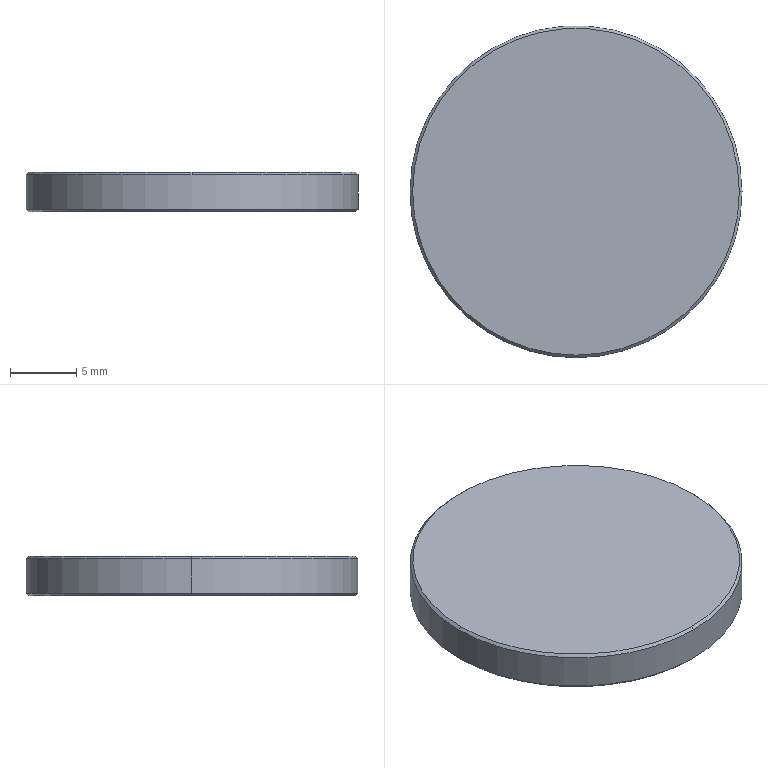Part | STEP file | TCHK-2D-D30-BB-TC-30X3.stp.STEP | 1 solid | 10 faces | box 25 x 25 x 3 mm | volume 1469 mm3 | cone 6 | plane 2 | cylinder 2 | commonest cylinder face diameters 25 x2
STEP:
#1=CARTESIAN_POINT('',(-12.3,0.,0.000000292));
#2=VERTEX_POINT('',#1);
#3=CARTESIAN_POINT('',(12.3,0.,0.000000292));
#4=VERTEX_POINT('',#3);
#5=CARTESIAN_POINT('',(0.,0.,0.000000292));
#6=DIRECTION('',(0.,0.,-1.));
#7=DIRECTION('',(-1.,0.,0.));
#8=AXIS2_PLACEMENT_3D('',#5,#6,#7);
#9=CIRCLE('',#8,12.3);
#10=EDGE_CURVE('',#2,#4,#9,.T.);
#11=ORIENTED_EDGE('',*,*,#10,.T.);
#12=CARTESIAN_POINT('',(0.,-12.3,0.000000292));
#13=VERTEX_POINT('',#12);
#14=CARTESIAN_POINT('',(0.,0.,0.000000292));
#15=DIRECTION('',(0.,0.,-1.));
#16=DIRECTION('',(1.,0.,0.));
#17=AXIS2_PLACEMENT_3D('',#14,#15,#16);
#18=CIRCLE('',#17,12.3);
#19=EDGE_CURVE('',#4,#13,#18,.T.);
#20=ORIENTED_EDGE('',*,*,#19,.T.);
#21=CARTESIAN_POINT('',(0.,0.,0.000000292));
#22=DIRECTION('',(0.,0.,-1.));
#23=DIRECTION('',(1.,0.,0.));
#24=AXIS2_PLACEMENT_3D('',#21,#22,#23);
#25=CIRCLE('',#24,12.3);
#26=EDGE_CURVE('',#13,#2,#25,.T.);
#27=ORIENTED_EDGE('',*,*,#26,.T.);
#28=EDGE_LOOP('',(#11,#20,#27));
#29=FACE_OUTER_BOUND('',#28,.T.);
#30=CARTESIAN_POINT('',(0.,0.,0.));
#31=DIRECTION('',(0.,0.,1.));
#32=DIRECTION('',(1.,0.,0.));
#33=AXIS2_PLACEMENT_3D('',#30,#31,#32);
#34=PLANE('',#33);
#35=ADVANCED_FACE('',(#29),#34,.F.);
#36=CARTESIAN_POINT('',(0.,-12.5,0.2));
#37=VERTEX_POINT('',#36);
#38=CARTESIAN_POINT('',(0.,-12.4,0.1));
#39=DIRECTION('',(0.,-0.7071,0.7071));
#40=VECTOR('',#39,1000.);
#41=LINE('',#38,#40);
#42=EDGE_CURVE('',#13,#37,#41,.T.);
#43=ORIENTED_EDGE('',*,*,#42,.F.);
#44=ORIENTED_EDGE('',*,*,#19,.F.);
#45=CARTESIAN_POINT('',(12.5,0.,0.2));
#46=VERTEX_POINT('',#45);
#47=CARTESIAN_POINT('',(12.3,0.000000002,0.000000547));
#48=DIRECTION('',(0.7071,-0.000000002,0.7071));
#49=VECTOR('',#48,1000.);
#50=LINE('',#47,#49);
#51=EDGE_CURVE('',#4,#46,#50,.T.);
#52=ORIENTED_EDGE('',*,*,#51,.T.);
#53=CARTESIAN_POINT('',(0.,0.,0.2));
#54=DIRECTION('',(0.,0.,-1.));
#55=DIRECTION('',(1.,0.,0.));
#56=AXIS2_PLACEMENT_3D('',#53,#54,#55);
#57=CIRCLE('',#56,12.5);
#58=EDGE_CURVE('',#46,#37,#57,.T.);
#59=ORIENTED_EDGE('',*,*,#58,.T.);
#60=EDGE_LOOP('',(#43,#44,#52,#59));
#61=FACE_OUTER_BOUND('',#60,.T.);
#62=CARTESIAN_POINT('',(0.,0.,0.1));
#63=DIRECTION('',(0.,0.,1.));
#64=DIRECTION('',(0.,-1.,0.));
#65=AXIS2_PLACEMENT_3D('',#62,#63,#64);
#66=CONICAL_SURFACE('',#65,12.4,0.7854);
#67=ADVANCED_FACE('',(#61),#66,.T.);
#68=CARTESIAN_POINT('',(-12.5,0.,0.2));
#69=VERTEX_POINT('',#68);
#70=CARTESIAN_POINT('',(-12.3,-0.000000002,0.000000547));
#71=DIRECTION('',(-0.7071,0.000000002,0.7071));
#72=VECTOR('',#71,1000.);
#73=LINE('',#70,#72);
#74=EDGE_CURVE('',#2,#69,#73,.T.);
#75=ORIENTED_EDGE('',*,*,#74,.T.);
#76=CARTESIAN_POINT('',(0.,0.,0.2));
#77=DIRECTION('',(0.,0.,-1.));
#78=DIRECTION('',(-1.,0.,0.));
#79=AXIS2_PLACEMENT_3D('',#76,#77,#78);
#80=CIRCLE('',#79,12.5);
#81=EDGE_CURVE('',#69,#46,#80,.T.);
#82=ORIENTED_EDGE('',*,*,#81,.T.);
#83=ORIENTED_EDGE('',*,*,#51,.F.);
#84=ORIENTED_EDGE('',*,*,#10,.F.);
#85=EDGE_LOOP('',(#75,#82,#83,#84));
#86=FACE_OUTER_BOUND('',#85,.T.);
#87=CARTESIAN_POINT('',(0.,0.,0.1));
#88=DIRECTION('',(0.,0.,1.));
#89=DIRECTION('',(0.,-1.,0.));
#90=AXIS2_PLACEMENT_3D('',#87,#88,#89);
#91=CONICAL_SURFACE('',#90,12.4,0.7854);
#92=ADVANCED_FACE('',(#86),#91,.T.);
#93=CARTESIAN_POINT('',(12.5,0.,2.8));
#94=VERTEX_POINT('',#93);
#95=CARTESIAN_POINT('',(12.5,0.000000001,0.2));
#96=DIRECTION('',(0.,0.,1.));
#97=VECTOR('',#96,1000.);
#98=LINE('',#95,#97);
#99=EDGE_CURVE('',#46,#94,#98,.T.);
#100=ORIENTED_EDGE('',*,*,#99,.F.);
#101=ORIENTED_EDGE('',*,*,#81,.F.);
#102=CARTESIAN_POINT('',(-12.5,0.,2.8));
#103=VERTEX_POINT('',#102);
#104=CARTESIAN_POINT('',(-12.5,-0.000000001,0.2));
#105=DIRECTION('',(0.,0.,1.));
#106=VECTOR('',#105,1000.);
#107=LINE('',#104,#106);
#108=EDGE_CURVE('',#69,#103,#107,.T.);
#109=ORIENTED_EDGE('',*,*,#108,.T.);
#110=CARTESIAN_POINT('',(0.,0.,2.8));
#111=DIRECTION('',(0.,0.,1.));
#112=DIRECTION('',(1.,0.,0.));
#113=AXIS2_PLACEMENT_3D('',#110,#111,#112);
#114=CIRCLE('',#113,12.5);
#115=EDGE_CURVE('',#94,#103,#114,.T.);
#116=ORIENTED_EDGE('',*,*,#115,.F.);
#117=EDGE_LOOP('',(#100,#101,#109,#116));
#118=FACE_OUTER_BOUND('',#117,.T.);
#119=CARTESIAN_POINT('',(0.,0.,0.));
#120=DIRECTION('',(0.,0.,1.));
#121=DIRECTION('',(1.,0.,0.));
#122=AXIS2_PLACEMENT_3D('',#119,#120,#121);
#123=CYLINDRICAL_SURFACE('',#122,12.5);
#124=ADVANCED_FACE('',(#118),#123,.T.);
#125=CARTESIAN_POINT('',(12.3,0.,3.));
#126=VERTEX_POINT('',#125);
#127=CARTESIAN_POINT('',(12.3,0.000000002,3.));
#128=DIRECTION('',(0.7071,-0.000000002,-0.7071));
#129=VECTOR('',#128,1000.);
#130=LINE('',#127,#129);
#131=EDGE_CURVE('',#126,#94,#130,.T.);
#132=ORIENTED_EDGE('',*,*,#131,.T.);
#133=ORIENTED_EDGE('',*,*,#115,.T.);
#134=CARTESIAN_POINT('',(-12.3,0.,3.));
#135=VERTEX_POINT('',#134);
#136=CARTESIAN_POINT('',(-12.3,-0.000000002,3.));
#137=DIRECTION('',(-0.7071,0.000000002,-0.7071));
#138=VECTOR('',#137,1000.);
#139=LINE('',#136,#138);
#140=EDGE_CURVE('',#135,#103,#139,.T.);
#141=ORIENTED_EDGE('',*,*,#140,.F.);
#142=CARTESIAN_POINT('',(0.,0.,3.));
#143=DIRECTION('',(0.,0.,1.));
#144=DIRECTION('',(1.,0.,0.));
#145=AXIS2_PLACEMENT_3D('',#142,#143,#144);
#146=CIRCLE('',#145,12.3);
#147=EDGE_CURVE('',#126,#135,#146,.T.);
#148=ORIENTED_EDGE('',*,*,#147,.F.);
#149=EDGE_LOOP('',(#132,#133,#141,#148));
#150=FACE_OUTER_BOUND('',#149,.T.);
#151=CARTESIAN_POINT('',(0.,0.,2.9));
#152=DIRECTION('',(0.,0.,-1.));
#153=DIRECTION('',(0.,-1.,0.));
#154=AXIS2_PLACEMENT_3D('',#151,#152,#153);
#155=CONICAL_SURFACE('',#154,12.4,0.7854);
#156=ADVANCED_FACE('',(#150),#155,.T.);
#157=ORIENTED_EDGE('',*,*,#147,.T.);
#158=CARTESIAN_POINT('',(0.,-12.3,3.));
#159=VERTEX_POINT('',#158);
#160=CARTESIAN_POINT('',(0.,0.,3.));
#161=DIRECTION('',(0.,0.,1.));
#162=DIRECTION('',(-1.,0.,0.));
#163=AXIS2_PLACEMENT_3D('',#160,#161,#162);
#164=CIRCLE('',#163,12.3);
#165=EDGE_CURVE('',#135,#159,#164,.T.);
#166=ORIENTED_EDGE('',*,*,#165,.T.);
#167=CARTESIAN_POINT('',(0.,0.,3.));
#168=DIRECTION('',(0.,0.,1.));
#169=DIRECTION('',(-1.,0.,0.));
#170=AXIS2_PLACEMENT_3D('',#167,#168,#169);
#171=CIRCLE('',#170,12.3);
#172=EDGE_CURVE('',#159,#126,#171,.T.);
#173=ORIENTED_EDGE('',*,*,#172,.T.);
#174=EDGE_LOOP('',(#157,#166,#173));
#175=FACE_OUTER_BOUND('',#174,.T.);
#176=CARTESIAN_POINT('',(0.,0.,3.));
#177=DIRECTION('',(0.,0.,1.));
#178=DIRECTION('',(1.,0.,0.));
#179=AXIS2_PLACEMENT_3D('',#176,#177,#178);
#180=PLANE('',#179);
#181=ADVANCED_FACE('',(#175),#180,.T.);
#182=CARTESIAN_POINT('',(0.,-12.5,2.8));
#183=VERTEX_POINT('',#182);
#184=CARTESIAN_POINT('',(0.,-12.4,2.9));
#185=DIRECTION('',(0.,-0.7071,-0.7071));
#186=VECTOR('',#185,1000.);
#187=LINE('',#184,#186);
#188=EDGE_CURVE('',#159,#183,#187,.T.);
#189=ORIENTED_EDGE('',*,*,#188,.F.);
#190=ORIENTED_EDGE('',*,*,#165,.F.);
#191=ORIENTED_EDGE('',*,*,#140,.T.);
#192=CARTESIAN_POINT('',(0.,0.,2.8));
#193=DIRECTION('',(0.,0.,1.));
#194=DIRECTION('',(-1.,0.,0.));
#195=AXIS2_PLACEMENT_3D('',#192,#193,#194);
#196=CIRCLE('',#195,12.5);
#197=EDGE_CURVE('',#103,#183,#196,.T.);
#198=ORIENTED_EDGE('',*,*,#197,.T.);
#199=EDGE_LOOP('',(#189,#190,#191,#198));
#200=FACE_OUTER_BOUND('',#199,.T.);
#201=CARTESIAN_POINT('',(0.,0.,2.9));
#202=DIRECTION('',(0.,0.,-1.));
#203=DIRECTION('',(0.,-1.,0.));
#204=AXIS2_PLACEMENT_3D('',#201,#202,#203);
#205=CONICAL_SURFACE('',#204,12.4,0.7854);
#206=ADVANCED_FACE('',(#200),#205,.T.);
#207=ORIENTED_EDGE('',*,*,#108,.F.);
#208=CARTESIAN_POINT('',(0.,0.,0.2));
#209=DIRECTION('',(0.,0.,-1.));
#210=DIRECTION('',(1.,0.,0.));
#211=AXIS2_PLACEMENT_3D('',#208,#209,#210);
#212=CIRCLE('',#211,12.5);
#213=EDGE_CURVE('',#37,#69,#212,.T.);
#214=ORIENTED_EDGE('',*,*,#213,.F.);
#215=ORIENTED_EDGE('',*,*,#58,.F.);
#216=ORIENTED_EDGE('',*,*,#99,.T.);
#217=CARTESIAN_POINT('',(0.,0.,2.8));
#218=DIRECTION('',(0.,0.,1.));
#219=DIRECTION('',(-1.,0.,0.));
#220=AXIS2_PLACEMENT_3D('',#217,#218,#219);
#221=CIRCLE('',#220,12.5);
#222=EDGE_CURVE('',#183,#94,#221,.T.);
#223=ORIENTED_EDGE('',*,*,#222,.F.);
#224=ORIENTED_EDGE('',*,*,#197,.F.);
#225=EDGE_LOOP('',(#207,#214,#215,#216,#223,#224));
#226=FACE_OUTER_BOUND('',#225,.T.);
#227=CARTESIAN_POINT('',(0.,0.,0.));
#228=DIRECTION('',(0.,0.,1.));
#229=DIRECTION('',(1.,0.,0.));
#230=AXIS2_PLACEMENT_3D('',#227,#228,#229);
#231=CYLINDRICAL_SURFACE('',#230,12.5);
#232=ADVANCED_FACE('',(#226),#231,.T.);
#233=ORIENTED_EDGE('',*,*,#172,.F.);
#234=ORIENTED_EDGE('',*,*,#188,.T.);
#235=ORIENTED_EDGE('',*,*,#222,.T.);
#236=ORIENTED_EDGE('',*,*,#131,.F.);
#237=EDGE_LOOP('',(#233,#234,#235,#236));
#238=FACE_OUTER_BOUND('',#237,.T.);
#239=CARTESIAN_POINT('',(0.,0.,2.9));
#240=DIRECTION('',(0.,0.,-1.));
#241=DIRECTION('',(0.,-1.,0.));
#242=AXIS2_PLACEMENT_3D('',#239,#240,#241);
#243=CONICAL_SURFACE('',#242,12.4,0.7854);
#244=ADVANCED_FACE('',(#238),#243,.T.);
#245=ORIENTED_EDGE('',*,*,#26,.F.);
#246=ORIENTED_EDGE('',*,*,#42,.T.);
#247=ORIENTED_EDGE('',*,*,#213,.T.);
#248=ORIENTED_EDGE('',*,*,#74,.F.);
#249=EDGE_LOOP('',(#245,#246,#247,#248));
#250=FACE_OUTER_BOUND('',#249,.T.);
#251=CARTESIAN_POINT('',(0.,0.,0.1));
#252=DIRECTION('',(0.,0.,1.));
#253=DIRECTION('',(0.,-1.,0.));
#254=AXIS2_PLACEMENT_3D('',#251,#252,#253);
#255=CONICAL_SURFACE('',#254,12.4,0.7854);
#256=ADVANCED_FACE('',(#250),#255,.T.);
#257=CLOSED_SHELL('',(#35,#67,#92,#124,#156,#181,#206,#232,#244,#256));
#258=MANIFOLD_SOLID_BREP('',#257);
#259=CARTESIAN_POINT('',(0.,0.,0.));
#260=DIRECTION('',(0.,0.,1.));
#261=DIRECTION('',(1.,0.,0.));
#262=AXIS2_PLACEMENT_3D('',#259,#260,#261);
#263=(LENGTH_UNIT()NAMED_UNIT(*)SI_UNIT(.MILLI.,.METRE.));
#264=UNCERTAINTY_MEASURE_WITH_UNIT(LENGTH_MEASURE(0.00001),#263,'','');
#265=(NAMED_UNIT(*)PLANE_ANGLE_UNIT()SI_UNIT($,.RADIAN.));
#266=(NAMED_UNIT(*)SI_UNIT($,.STERADIAN.)SOLID_ANGLE_UNIT());
#267=(GEOMETRIC_REPRESENTATION_CONTEXT(3)GLOBAL_UNCERTAINTY_ASSIGNED_CONTEXT((#264))GLOBAL_UNIT_ASSIGNED_CONTEXT((#263,#265,#266))REPRESENTATION_CONTEXT('',''));
#268=ADVANCED_BREP_SHAPE_REPRESENTATION('',(#258,#262),#267);